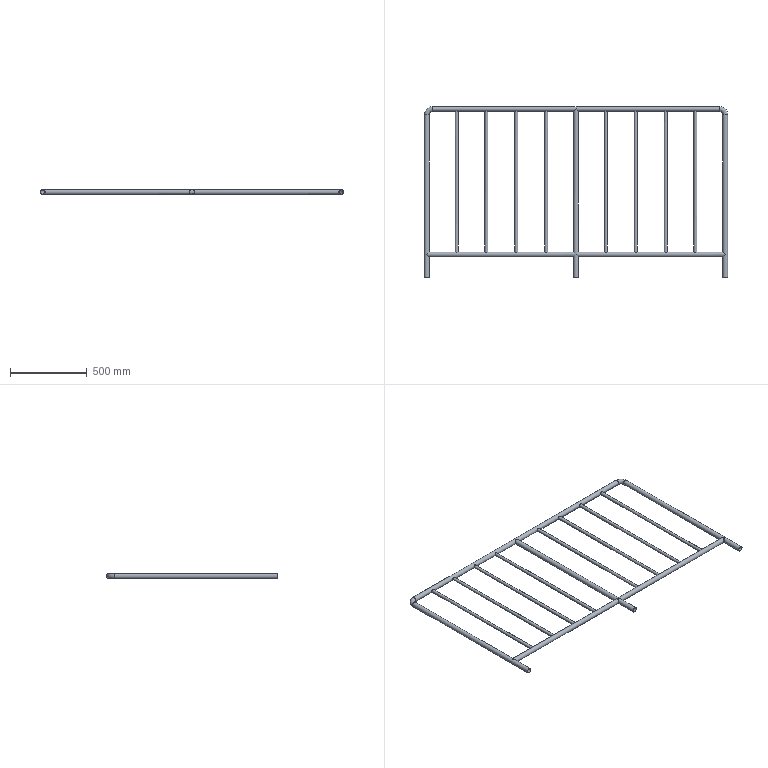Part | STEP file | 304 guardrail 1950X1100-D body_Default<As Machined> | 16 solids | 64 faces | box 1982 x 1116 x 32 mm | volume 1461752 mm3 | cylinder 49 | plane 11 | torus 4 | commonest cylinder face diameters 32 x27 18 x8 20 x8 29 x6